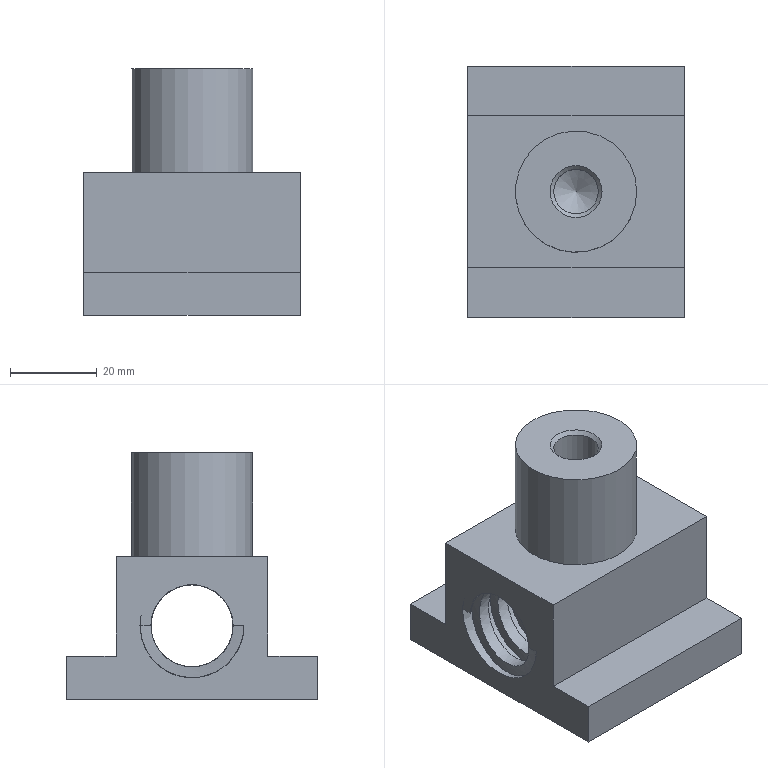Part | NX | features DATUM_CSYS 3, SKETCH 3, EXTRUDE 2, HOLE PACKAGE 2, SIMPLE HOLE 2, BLOCK 1, DATUM_ON_PATH 1, HELIX 1, SKIN 1, SUBTRACT 1, SYMBOLIC_THREAD 1 | 1 solid | 18 faces | box 50.001 x 58 x 57 mm | volume 63589 mm3 | plane 11 | cylinder 3 | cone 2 | spline 2 | commonest cylinder face diameters 10.3 x1 19 x1 28 x1